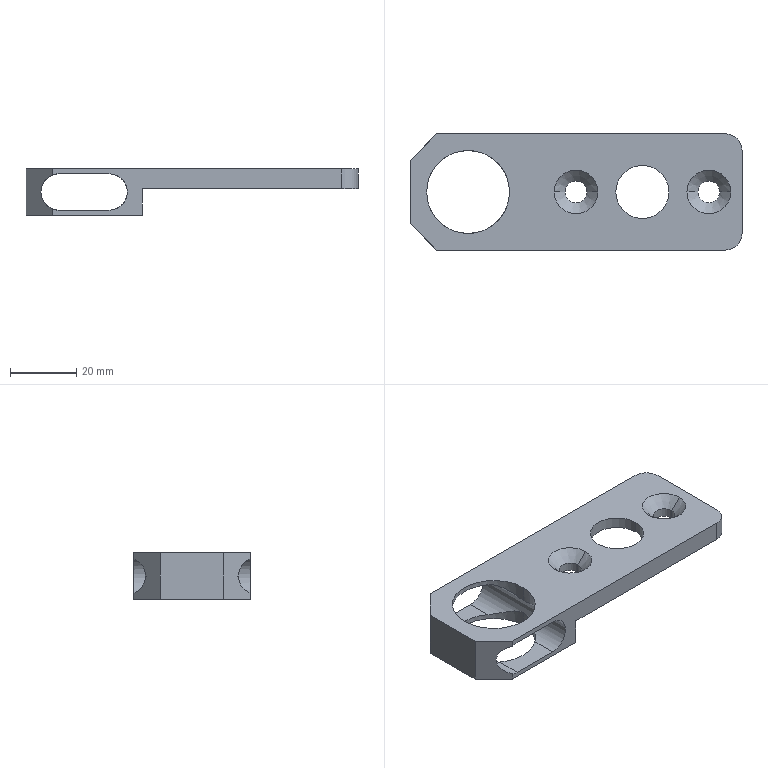Part | STEP file | Adjusting wrench QY-1-14 | 1 solid | 36 faces | box 100 x 35 x 14 mm | volume 16527 mm3 | cylinder 17 | plane 15 | cone 4 | commonest cylinder face diameters 25 x6 6.6 x4 11 x3 10 x2 16 x2